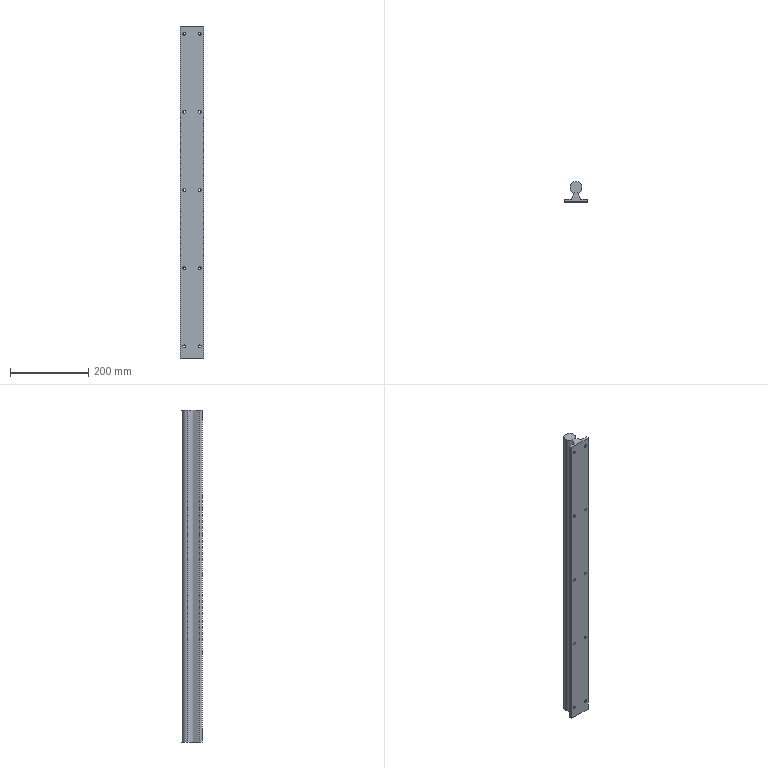Part | STEP file | 1 solid | 32 faces | box 60 x 52 x 850 mm | volume 1179797 mm3 | cylinder 23 | plane 9 | commonest cylinder face diameters 6.6 x20 30 x3